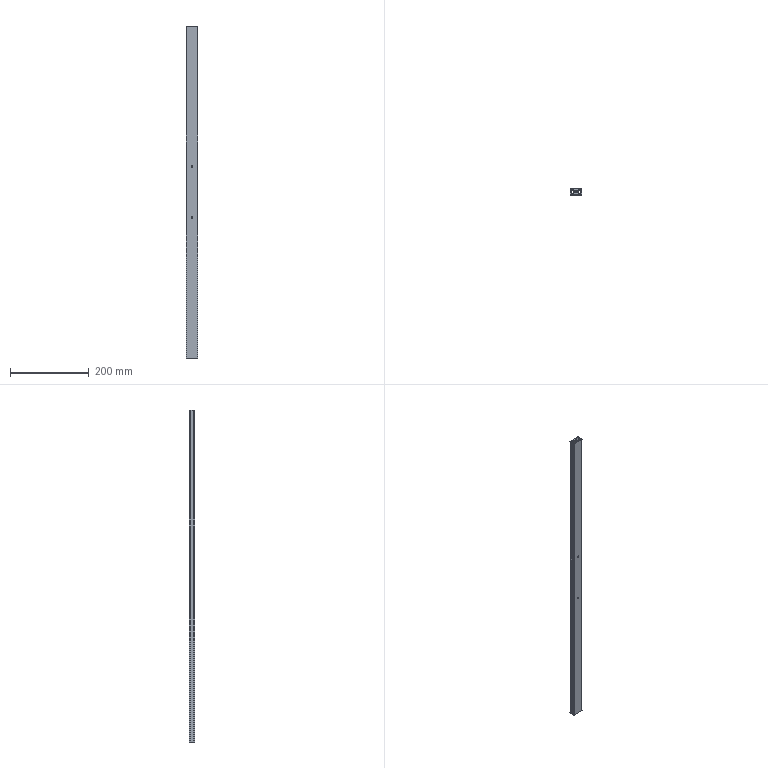Part | SolidWorks | features HoleWzd 2, BaseBody 1, MoveFace 1 | 1 solid | 117 faces | box 30 x 15 x 842 mm | volume 202454 mm3 | cylinder 59 | plane 46 | cone 12 | commonest cylinder face diameters 5 x17 3.3 x16 4.5 x16 1 x6 2 x4